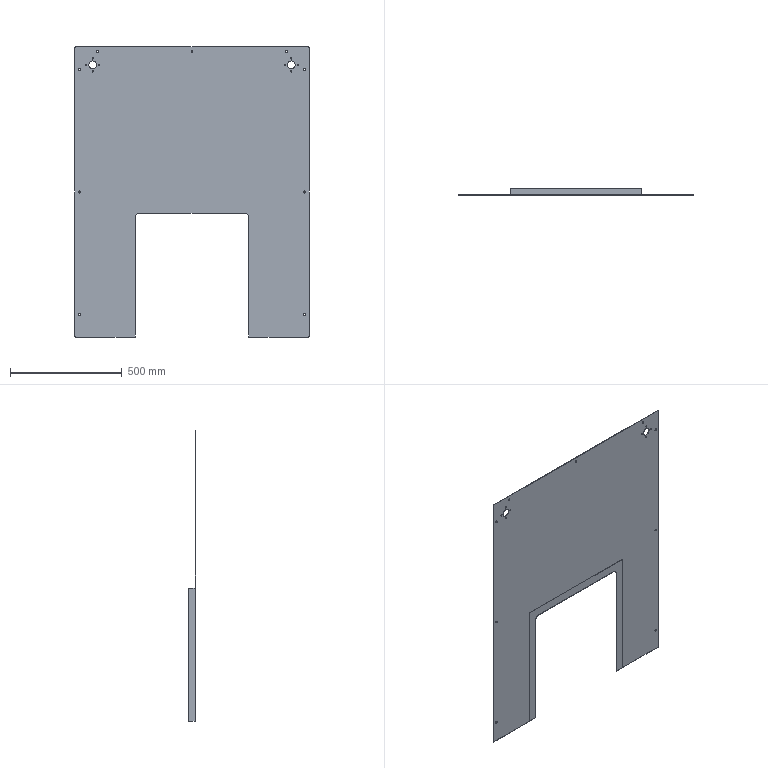Part | SolidWorks | features Fillet 2, FlatPattern 2, ICE 2, SMBaseFlange 2, SheetMetal 2, Cut 1, MirrorPattern 1 | 2 solids | 64 faces | box 1050 x 31.5 x 1300 mm | volume 1699042 mm3 | cylinder 44 | plane 20 | commonest cylinder face diameters 9 x18 6 x16 8 x4 35 x4 40 x2